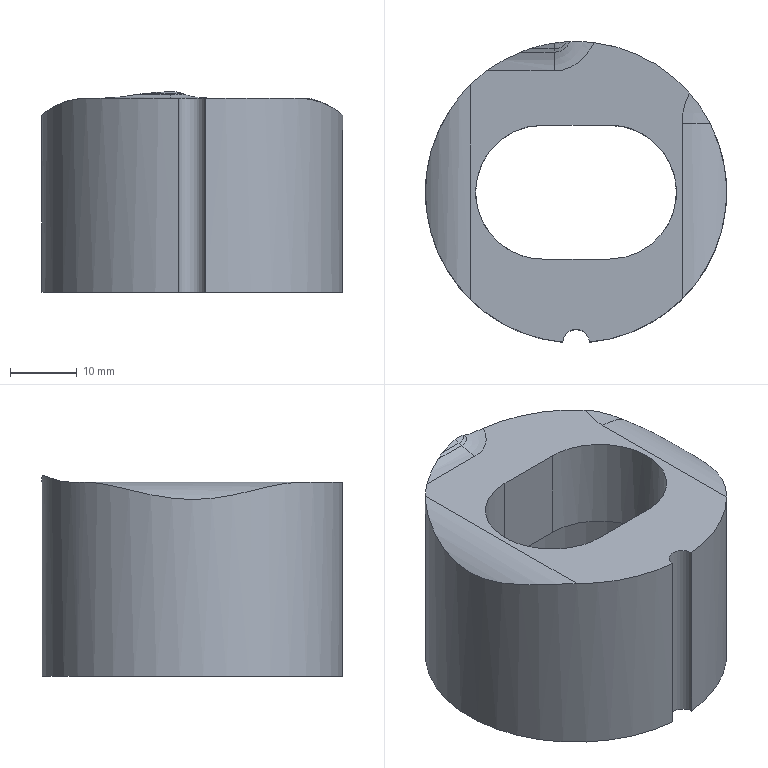Part | NX | features solid 2 | 1 solid | 19 faces | box 45 x 44.911 x 29.98 mm | volume 23323 mm3 | cylinder 10 | plane 6 | spline 3 | commonest cylinder face diameters 20 x3 12 x2 4 x1 15.009 x1 20.004 x1 36 x1
STEP:
#1=CARTESIAN_POINT('',(615.,-208.,21.));
#2=VERTEX_POINT('',#1);
#3=CARTESIAN_POINT('',(615.,-208.,35.));
#4=VERTEX_POINT('',#3);
#5=CARTESIAN_POINT('',(615.,-208.,-244.));
#6=DIRECTION('',(0.,0.,1.));
#7=VECTOR('',#6,1000.);
#8=LINE('',#5,#7);
#9=EDGE_CURVE('',#2,#4,#8,.T.);
#10=ORIENTED_EDGE('',*,*,#9,.T.);
#11=CARTESIAN_POINT('',(625.,-208.,35.));
#12=VERTEX_POINT('',#11);
#13=CARTESIAN_POINT('',(615.,-208.,35.));
#14=CARTESIAN_POINT('',(618.333,-208.,35.));
#15=CARTESIAN_POINT('',(621.666,-208.,35.));
#16=CARTESIAN_POINT('',(625.,-208.,35.));
#17=B_SPLINE_CURVE_WITH_KNOTS('',3,(#13,#14,#15,#16),.UNSPECIFIED.,.F.,.F.,(4,4),(0.,1.),.UNSPECIFIED.);
#18=EDGE_CURVE('',#4,#12,#17,.T.);
#19=ORIENTED_EDGE('',*,*,#18,.T.);
#20=CARTESIAN_POINT('',(625.,-208.,21.));
#21=VERTEX_POINT('',#20);
#22=CARTESIAN_POINT('',(625.,-208.,-244.));
#23=DIRECTION('',(0.,0.,1.));
#24=VECTOR('',#23,1000.);
#25=LINE('',#22,#24);
#26=EDGE_CURVE('',#21,#12,#25,.T.);
#27=ORIENTED_EDGE('',*,*,#26,.F.);
#28=CARTESIAN_POINT('',(615.,-208.,21.));
#29=DIRECTION('',(-1.,0.,0.));
#30=VECTOR('',#29,1000.);
#31=LINE('',#28,#30);
#32=EDGE_CURVE('',#21,#2,#31,.T.);
#33=ORIENTED_EDGE('',*,*,#32,.T.);
#34=EDGE_LOOP('',(#10,#19,#27,#33));
#35=FACE_BOUND('',#34,.T.);
#36=CARTESIAN_POINT('',(615.,-208.,-244.));
#37=DIRECTION('',(0.,1.,0.));
#38=DIRECTION('',(0.,0.,1.));
#39=AXIS2_PLACEMENT_3D('',#36,#37,#38);
#40=PLANE('',#39);
#41=ADVANCED_FACE('',(#35),#40,.T.);
#42=CARTESIAN_POINT('',(625.,-188.,35.));
#43=VERTEX_POINT('',#42);
#44=CARTESIAN_POINT('',(625.,-208.,35.));
#45=CARTESIAN_POINT('',(625.109,-207.999,35.));
#46=CARTESIAN_POINT('',(625.233,-207.998,35.));
#47=CARTESIAN_POINT('',(625.579,-207.987,35.));
#48=CARTESIAN_POINT('',(626.137,-207.945,35.));
#49=CARTESIAN_POINT('',(626.956,-207.826,35.));
#50=CARTESIAN_POINT('',(627.896,-207.589,35.));
#51=CARTESIAN_POINT('',(629.14,-207.143,35.));
#52=CARTESIAN_POINT('',(630.59,-206.373,35.));
#53=CARTESIAN_POINT('',(632.622,-204.701,35.));
#54=CARTESIAN_POINT('',(634.479,-201.929,35.));
#55=CARTESIAN_POINT('',(635.26,-198.,35.));
#56=CARTESIAN_POINT('',(634.479,-194.072,35.));
#57=CARTESIAN_POINT('',(632.622,-191.299,35.));
#58=CARTESIAN_POINT('',(630.591,-189.628,35.));
#59=CARTESIAN_POINT('',(629.14,-188.857,35.));
#60=CARTESIAN_POINT('',(627.898,-188.411,35.));
#61=CARTESIAN_POINT('',(626.956,-188.174,35.));
#62=CARTESIAN_POINT('',(626.137,-188.055,35.));
#63=CARTESIAN_POINT('',(625.579,-188.013,35.));
#64=CARTESIAN_POINT('',(625.233,-188.004,35.));
#65=CARTESIAN_POINT('',(625.109,-188.002,35.));
#66=CARTESIAN_POINT('',(625.,-188.,35.));
#67=B_SPLINE_CURVE_WITH_KNOTS('',3,(#44,#45,#46,#47,#48,#49,#50,#51,#52,#53,#54,#55,#56,#57,#58,#59,#60,#61,#62,#63,#64,#65,#66),.UNSPECIFIED.,.F.,.F.,(4,1,1,1,1,1,1,1,1,1,1,1,1,1,1,1,1,1,1,1,4),(0.,0.007812,0.01562,0.03125,0.0625,0.09375,0.125,0.1875,0.25,0.375,0.5,0.625,0.75,0.8125,0.875,0.9062,0.9375,0.9687,0.9844,0.9922,1.),.UNSPECIFIED.);
#68=EDGE_CURVE('',#43,#12,#67,.F.);
#69=ORIENTED_EDGE('',*,*,#68,.F.);
#70=CARTESIAN_POINT('',(625.,-188.,21.));
#71=VERTEX_POINT('',#70);
#72=CARTESIAN_POINT('',(625.,-188.,-244.));
#73=DIRECTION('',(0.,0.,1.));
#74=VECTOR('',#73,1000.);
#75=LINE('',#72,#74);
#76=EDGE_CURVE('',#71,#43,#75,.T.);
#77=ORIENTED_EDGE('',*,*,#76,.F.);
#78=CARTESIAN_POINT('',(625.,-198.,21.));
#79=DIRECTION('',(0.,0.,-1.));
#80=DIRECTION('',(-1.,0.,0.));
#81=AXIS2_PLACEMENT_3D('',#78,#79,#80);
#82=CIRCLE('',#81,10.);
#83=EDGE_CURVE('',#21,#71,#82,.F.);
#84=ORIENTED_EDGE('',*,*,#83,.F.);
#85=ORIENTED_EDGE('',*,*,#26,.T.);
#86=EDGE_LOOP('',(#69,#77,#84,#85));
#87=FACE_BOUND('',#86,.T.);
#88=CARTESIAN_POINT('',(625.,-198.,-244.));
#89=DIRECTION('',(0.,0.,1.));
#90=DIRECTION('',(-1.,0.,0.));
#91=AXIS2_PLACEMENT_3D('',#88,#89,#90);
#92=CYLINDRICAL_SURFACE('',#91,10.);
#93=ADVANCED_FACE('',(#87),#92,.F.);
#94=CARTESIAN_POINT('',(615.,-188.,35.));
#95=VERTEX_POINT('',#94);
#96=CARTESIAN_POINT('',(615.,-188.,35.));
#97=CARTESIAN_POINT('',(618.333,-188.,35.));
#98=CARTESIAN_POINT('',(621.666,-188.,35.));
#99=CARTESIAN_POINT('',(625.,-188.,35.));
#100=B_SPLINE_CURVE_WITH_KNOTS('',3,(#96,#97,#98,#99),.UNSPECIFIED.,.F.,.F.,(4,4),(0.,1.),.UNSPECIFIED.);
#101=EDGE_CURVE('',#95,#43,#100,.T.);
#102=ORIENTED_EDGE('',*,*,#101,.F.);
#103=CARTESIAN_POINT('',(615.,-188.,21.));
#104=VERTEX_POINT('',#103);
#105=CARTESIAN_POINT('',(615.,-188.,-244.));
#106=DIRECTION('',(0.,0.,1.));
#107=VECTOR('',#106,1000.);
#108=LINE('',#105,#107);
#109=EDGE_CURVE('',#104,#95,#108,.T.);
#110=ORIENTED_EDGE('',*,*,#109,.F.);
#111=CARTESIAN_POINT('',(615.,-188.,21.));
#112=DIRECTION('',(-1.,0.,0.));
#113=VECTOR('',#112,1000.);
#114=LINE('',#111,#113);
#115=EDGE_CURVE('',#71,#104,#114,.T.);
#116=ORIENTED_EDGE('',*,*,#115,.F.);
#117=ORIENTED_EDGE('',*,*,#76,.T.);
#118=EDGE_LOOP('',(#102,#110,#116,#117));
#119=FACE_BOUND('',#118,.T.);
#120=CARTESIAN_POINT('',(615.,-188.,-244.));
#121=DIRECTION('',(0.,1.,0.));
#122=DIRECTION('',(0.,0.,1.));
#123=AXIS2_PLACEMENT_3D('',#120,#121,#122);
#124=PLANE('',#123);
#125=ADVANCED_FACE('',(#119),#124,.F.);
#126=CARTESIAN_POINT('',(615.,-188.,35.));
#127=CARTESIAN_POINT('',(614.891,-188.001,35.));
#128=CARTESIAN_POINT('',(614.767,-188.002,35.));
#129=CARTESIAN_POINT('',(614.421,-188.013,35.));
#130=CARTESIAN_POINT('',(613.863,-188.055,35.));
#131=CARTESIAN_POINT('',(613.044,-188.174,35.));
#132=CARTESIAN_POINT('',(612.103,-188.411,35.));
#133=CARTESIAN_POINT('',(610.859,-188.857,35.));
#134=CARTESIAN_POINT('',(609.41,-189.627,35.));
#135=CARTESIAN_POINT('',(607.377,-191.299,35.));
#136=CARTESIAN_POINT('',(605.521,-194.071,35.));
#137=CARTESIAN_POINT('',(604.74,-198.,35.));
#138=CARTESIAN_POINT('',(605.52,-201.928,35.));
#139=CARTESIAN_POINT('',(607.378,-204.701,35.));
#140=CARTESIAN_POINT('',(609.409,-206.372,35.));
#141=CARTESIAN_POINT('',(610.86,-207.143,35.));
#142=CARTESIAN_POINT('',(612.102,-207.589,35.));
#143=CARTESIAN_POINT('',(613.044,-207.826,35.));
#144=CARTESIAN_POINT('',(613.863,-207.945,35.));
#145=CARTESIAN_POINT('',(614.421,-207.987,35.));
#146=CARTESIAN_POINT('',(614.767,-207.996,35.));
#147=CARTESIAN_POINT('',(614.891,-207.998,35.));
#148=CARTESIAN_POINT('',(615.,-208.,35.));
#149=B_SPLINE_CURVE_WITH_KNOTS('',3,(#126,#127,#128,#129,#130,#131,#132,#133,#134,#135,#136,#137,#138,#139,#140,#141,#142,#143,#144,#145,#146,#147,#148),.UNSPECIFIED.,.F.,.F.,(4,1,1,1,1,1,1,1,1,1,1,1,1,1,1,1,1,1,1,1,4),(0.,0.007812,0.01562,0.03125,0.0625,0.09375,0.125,0.1875,0.25,0.375,0.5,0.625,0.75,0.8125,0.875,0.9062,0.9375,0.9687,0.9844,0.9922,1.),.UNSPECIFIED.);
#150=EDGE_CURVE('',#4,#95,#149,.F.);
#151=ORIENTED_EDGE('',*,*,#150,.F.);
#152=ORIENTED_EDGE('',*,*,#9,.F.);
#153=CARTESIAN_POINT('',(615.,-198.,21.));
#154=DIRECTION('',(0.,0.,-1.));
#155=DIRECTION('',(-1.,0.,0.));
#156=AXIS2_PLACEMENT_3D('',#153,#154,#155);
#157=CIRCLE('',#156,10.);
#158=EDGE_CURVE('',#104,#2,#157,.F.);
#159=ORIENTED_EDGE('',*,*,#158,.F.);
#160=ORIENTED_EDGE('',*,*,#109,.T.);
#161=EDGE_LOOP('',(#151,#152,#159,#160));
#162=FACE_BOUND('',#161,.T.);
#163=CARTESIAN_POINT('',(615.,-198.,-244.));
#164=DIRECTION('',(0.,0.,1.));
#165=DIRECTION('',(-1.,0.,0.));
#166=AXIS2_PLACEMENT_3D('',#163,#164,#165);
#167=CYLINDRICAL_SURFACE('',#166,10.);
#168=ADVANCED_FACE('',(#162),#167,.F.);
#169=CARTESIAN_POINT('',(618.002,-220.411,6.));
#170=VERTEX_POINT('',#169);
#171=CARTESIAN_POINT('',(621.998,-220.411,6.));
#172=VERTEX_POINT('',#171);
#173=CARTESIAN_POINT('',(620.,-198.,6.));
#174=DIRECTION('',(0.,0.,-1.));
#175=DIRECTION('',(-1.,0.,0.));
#176=AXIS2_PLACEMENT_3D('',#173,#174,#175);
#177=CIRCLE('',#176,22.5);
#178=EDGE_CURVE('',#170,#172,#177,.T.);
#179=ORIENTED_EDGE('',*,*,#178,.T.);
#180=CARTESIAN_POINT('',(620.,-220.5,6.));
#181=DIRECTION('',(0.,0.,-1.));
#182=DIRECTION('',(0.,1.,0.));
#183=AXIS2_PLACEMENT_3D('',#180,#181,#182);
#184=CIRCLE('',#183,2.);
#185=EDGE_CURVE('',#170,#172,#184,.T.);
#186=ORIENTED_EDGE('',*,*,#185,.F.);
#187=EDGE_LOOP('',(#179,#186));
#188=FACE_BOUND('',#187,.T.);
#189=CARTESIAN_POINT('',(602.,-198.,6.));
#190=VERTEX_POINT('',#189);
#191=CARTESIAN_POINT('',(620.,-198.,6.));
#192=DIRECTION('',(0.,0.,-1.));
#193=DIRECTION('',(-1.,0.,0.));
#194=AXIS2_PLACEMENT_3D('',#191,#192,#193);
#195=CIRCLE('',#194,18.);
#196=EDGE_CURVE('',#190,#190,#195,.F.);
#197=ORIENTED_EDGE('',*,*,#196,.T.);
#198=EDGE_LOOP('',(#197));
#199=FACE_BOUND('',#198,.T.);
#200=CARTESIAN_POINT('',(620.,-198.,6.));
#201=DIRECTION('',(0.,0.,1.));
#202=DIRECTION('',(-1.,0.,0.));
#203=AXIS2_PLACEMENT_3D('',#200,#201,#202);
#204=PLANE('',#203);
#205=ADVANCED_FACE('',(#188,#199),#204,.F.);
#206=CARTESIAN_POINT('',(636.941,-183.193,35.));
#207=VERTEX_POINT('',#206);
#208=CARTESIAN_POINT('',(640.057,-187.804,34.071));
#209=VERTEX_POINT('',#208);
#210=CARTESIAN_POINT('',(636.941,-183.193,35.));
#211=CARTESIAN_POINT('',(638.198,-184.631,35.));
#212=CARTESIAN_POINT('',(639.217,-186.152,34.461));
#213=CARTESIAN_POINT('',(640.057,-187.804,34.069));
#214=B_SPLINE_CURVE_WITH_KNOTS('',3,(#210,#211,#212,#213),.UNSPECIFIED.,.F.,.F.,(4,4),(0.,0.005644),.UNSPECIFIED.);
#215=EDGE_CURVE('',#207,#209,#214,.T.);
#216=ORIENTED_EDGE('',*,*,#215,.T.);
#217=CARTESIAN_POINT('',(635.855,-213.965,35.));
#218=VERTEX_POINT('',#217);
#219=CARTESIAN_POINT('',(640.057,-187.804,34.072));
#220=CARTESIAN_POINT('',(641.122,-189.898,33.578));
#221=CARTESIAN_POINT('',(642.209,-193.22,32.737));
#222=CARTESIAN_POINT('',(642.597,-198.006,32.381));
#223=CARTESIAN_POINT('',(642.208,-202.794,32.741));
#224=CARTESIAN_POINT('',(640.362,-208.398,34.158));
#225=CARTESIAN_POINT('',(637.569,-212.262,35.));
#226=CARTESIAN_POINT('',(635.855,-213.964,35.));
#227=B_SPLINE_CURVE_WITH_KNOTS('',3,(#219,#220,#221,#222,#223,#224,#225,#226),.UNSPECIFIED.,.F.,.F.,(4,1,1,1,1,4),(0.0003348,0.007451,0.01101,0.01457,0.02168,0.0288),.UNSPECIFIED.);
#228=EDGE_CURVE('',#209,#218,#227,.T.);
#229=ORIENTED_EDGE('',*,*,#228,.T.);
#230=CARTESIAN_POINT('',(621.998,-220.411,35.));
#231=VERTEX_POINT('',#230);
#232=CARTESIAN_POINT('',(620.,-198.,35.));
#233=DIRECTION('',(0.,0.,-1.));
#234=DIRECTION('',(-1.,0.,0.));
#235=AXIS2_PLACEMENT_3D('',#232,#233,#234);
#236=CIRCLE('',#235,22.5);
#237=EDGE_CURVE('',#231,#218,#236,.F.);
#238=ORIENTED_EDGE('',*,*,#237,.F.);
#239=CARTESIAN_POINT('',(621.998,-220.411,21.));
#240=DIRECTION('',(0.,0.,-1.));
#241=VECTOR('',#240,1000.);
#242=LINE('',#239,#241);
#243=EDGE_CURVE('',#172,#231,#242,.F.);
#244=ORIENTED_EDGE('',*,*,#243,.F.);
#245=ORIENTED_EDGE('',*,*,#178,.F.);
#246=CARTESIAN_POINT('',(618.002,-220.411,35.));
#247=VERTEX_POINT('',#246);
#248=CARTESIAN_POINT('',(618.002,-220.411,21.));
#249=DIRECTION('',(0.,0.,-1.));
#250=VECTOR('',#249,1000.);
#251=LINE('',#248,#250);
#252=EDGE_CURVE('',#247,#170,#251,.T.);
#253=ORIENTED_EDGE('',*,*,#252,.F.);
#254=CARTESIAN_POINT('',(604.208,-214.028,35.));
#255=VERTEX_POINT('',#254);
#256=CARTESIAN_POINT('',(620.,-198.,35.));
#257=DIRECTION('',(0.,0.,-1.));
#258=DIRECTION('',(-1.,0.,0.));
#259=AXIS2_PLACEMENT_3D('',#256,#257,#258);
#260=CIRCLE('',#259,22.5);
#261=EDGE_CURVE('',#255,#247,#260,.F.);
#262=ORIENTED_EDGE('',*,*,#261,.F.);
#263=CARTESIAN_POINT('',(604.208,-181.972,35.));
#264=VERTEX_POINT('',#263);
#265=CARTESIAN_POINT('',(604.208,-214.028,35.));
#266=CARTESIAN_POINT('',(602.043,-211.894,35.));
#267=CARTESIAN_POINT('',(599.551,-208.158,34.001));
#268=CARTESIAN_POINT('',(597.807,-202.515,32.71));
#269=CARTESIAN_POINT('',(597.347,-198.025,32.27));
#270=CARTESIAN_POINT('',(597.802,-193.506,32.705));
#271=CARTESIAN_POINT('',(599.546,-187.85,34.));
#272=CARTESIAN_POINT('',(602.043,-184.106,35.));
#273=CARTESIAN_POINT('',(604.208,-181.972,35.));
#274=B_SPLINE_CURVE_WITH_KNOTS('',3,(#265,#266,#267,#268,#269,#270,#271,#272,#273),.UNSPECIFIED.,.F.,.F.,(4,1,1,1,1,1,4),(0.,0.009016,0.01352,0.01803,0.02254,0.02705,0.03606),.UNSPECIFIED.);
#275=EDGE_CURVE('',#255,#264,#274,.T.);
#276=ORIENTED_EDGE('',*,*,#275,.T.);
#277=CARTESIAN_POINT('',(606.645,-179.892,35.));
#278=VERTEX_POINT('',#277);
#279=CARTESIAN_POINT('',(620.,-198.,35.));
#280=DIRECTION('',(0.,0.,-1.));
#281=DIRECTION('',(-1.,0.,0.));
#282=AXIS2_PLACEMENT_3D('',#279,#280,#281);
#283=CIRCLE('',#282,22.5);
#284=EDGE_CURVE('',#278,#264,#283,.F.);
#285=ORIENTED_EDGE('',*,*,#284,.F.);
#286=CARTESIAN_POINT('',(611.709,-177.083,35.546));
#287=VERTEX_POINT('',#286);
#288=CARTESIAN_POINT('',(611.709,-177.083,35.546));
#289=CARTESIAN_POINT('',(609.909,-177.797,35.258));
#290=CARTESIAN_POINT('',(608.225,-178.727,35.));
#291=CARTESIAN_POINT('',(606.645,-179.892,35.));
#292=B_SPLINE_CURVE_WITH_KNOTS('',3,(#288,#289,#290,#291),.UNSPECIFIED.,.F.,.F.,(4,4),(0.,0.005817),.UNSPECIFIED.);
#293=EDGE_CURVE('',#287,#278,#292,.T.);
#294=ORIENTED_EDGE('',*,*,#293,.F.);
#295=CARTESIAN_POINT('',(613.191,-176.555,35.731));
#296=VERTEX_POINT('',#295);
#297=CARTESIAN_POINT('',(611.709,-177.083,35.546));
#298=CARTESIAN_POINT('',(612.194,-176.891,35.624));
#299=CARTESIAN_POINT('',(612.688,-176.715,35.683));
#300=CARTESIAN_POINT('',(613.191,-176.555,35.731));
#301=B_SPLINE_CURVE_WITH_KNOTS('',3,(#297,#298,#299,#300),.UNSPECIFIED.,.F.,.F.,(4,4),(0.006984,0.008558),.UNSPECIFIED.);
#302=EDGE_CURVE('',#287,#296,#301,.T.);
#303=ORIENTED_EDGE('',*,*,#302,.T.);
#304=CARTESIAN_POINT('',(616.734,-175.738,35.975));
#305=VERTEX_POINT('',#304);
#306=CARTESIAN_POINT('',(620.,-198.,29.318));
#307=DIRECTION('',(0.,-0.2865,0.9581));
#308=DIRECTION('',(0.,0.9581,0.2865));
#309=AXIS2_PLACEMENT_3D('',#306,#307,#308);
#310=ELLIPSE('',#309,23.485,22.5);
#311=EDGE_CURVE('',#296,#305,#310,.F.);
#312=ORIENTED_EDGE('',*,*,#311,.T.);
#313=CARTESIAN_POINT('',(618.619,-175.542,35.718));
#314=VERTEX_POINT('',#313);
#315=CARTESIAN_POINT('',(618.622,-175.542,35.716));
#316=CARTESIAN_POINT('',(618.016,-175.579,35.915));
#317=CARTESIAN_POINT('',(617.374,-175.644,36.003));
#318=CARTESIAN_POINT('',(616.734,-175.738,35.975));
#319=B_SPLINE_CURVE_WITH_KNOTS('',3,(#315,#316,#317,#318),.UNSPECIFIED.,.F.,.F.,(4,4),(0.002426,0.00434),.UNSPECIFIED.);
#320=EDGE_CURVE('',#314,#305,#319,.T.);
#321=ORIENTED_EDGE('',*,*,#320,.F.);
#322=CARTESIAN_POINT('',(619.085,-175.519,35.523));
#323=VERTEX_POINT('',#322);
#324=CARTESIAN_POINT('',(619.085,-175.519,35.523));
#325=CARTESIAN_POINT('',(618.927,-175.525,35.586));
#326=CARTESIAN_POINT('',(618.777,-175.533,35.666));
#327=CARTESIAN_POINT('',(618.617,-175.543,35.719));
#328=B_SPLINE_CURVE_WITH_KNOTS('',3,(#324,#325,#326,#327),.UNSPECIFIED.,.F.,.F.,(4,4),(0.,0.0005083),.UNSPECIFIED.);
#329=EDGE_CURVE('',#323,#314,#328,.T.);
#330=ORIENTED_EDGE('',*,*,#329,.F.);
#331=CARTESIAN_POINT('',(622.733,-175.667,35.));
#332=VERTEX_POINT('',#331);
#333=CARTESIAN_POINT('',(622.733,-175.667,35.));
#334=CARTESIAN_POINT('',(622.118,-175.591,35.));
#335=CARTESIAN_POINT('',(620.888,-175.492,35.073));
#336=CARTESIAN_POINT('',(619.655,-175.495,35.276));
#337=CARTESIAN_POINT('',(619.085,-175.519,35.523));
#338=B_SPLINE_CURVE_WITH_KNOTS('',3,(#333,#334,#335,#336,#337),.UNSPECIFIED.,.F.,.F.,(4,1,4),(0.,0.001854,0.003709),.UNSPECIFIED.);
#339=EDGE_CURVE('',#332,#323,#338,.T.);
#340=ORIENTED_EDGE('',*,*,#339,.F.);
#341=CARTESIAN_POINT('',(620.,-198.,35.));
#342=DIRECTION('',(0.,0.,-1.));
#343=DIRECTION('',(-1.,0.,0.));
#344=AXIS2_PLACEMENT_3D('',#341,#342,#343);
#345=CIRCLE('',#344,22.5);
#346=EDGE_CURVE('',#207,#332,#345,.F.);
#347=ORIENTED_EDGE('',*,*,#346,.F.);
#348=EDGE_LOOP('',(#216,#229,#238,#244,#245,#253,#262,#276,#285,#294,#303,#312,#321,#330,#340,#347));
#349=FACE_BOUND('',#348,.T.);
#350=CARTESIAN_POINT('',(620.,-198.,6.));
#351=DIRECTION('',(0.,0.,1.));
#352=DIRECTION('',(-1.,0.,0.));
#353=AXIS2_PLACEMENT_3D('',#350,#351,#352);
#354=CYLINDRICAL_SURFACE('',#353,22.5);
#355=ADVANCED_FACE('',(#349),#354,.T.);
#356=CARTESIAN_POINT('',(602.,-198.,21.));
#357=VERTEX_POINT('',#356);
#358=CARTESIAN_POINT('',(620.,-198.,21.));
#359=DIRECTION('',(0.,0.,-1.));
#360=DIRECTION('',(-1.,0.,0.));
#361=AXIS2_PLACEMENT_3D('',#358,#359,#360);
#362=CIRCLE('',#361,18.);
#363=EDGE_CURVE('',#357,#357,#362,.T.);
#364=ORIENTED_EDGE('',*,*,#363,.F.);
#365=EDGE_LOOP('',(#364));
#366=FACE_BOUND('',#365,.T.);
#367=ORIENTED_EDGE('',*,*,#196,.F.);
#368=EDGE_LOOP('',(#367));
#369=FACE_BOUND('',#368,.T.);
#370=CARTESIAN_POINT('',(620.,-198.,28.));
#371=DIRECTION('',(0.,0.,-1.));
#372=DIRECTION('',(1.,0.,0.));
#373=AXIS2_PLACEMENT_3D('',#370,#371,#372);
#374=CYLINDRICAL_SURFACE('',#373,18.);
#375=ADVANCED_FACE('',(#366,#369),#374,.F.);
#376=ORIENTED_EDGE('',*,*,#32,.F.);
#377=ORIENTED_EDGE('',*,*,#83,.T.);
#378=ORIENTED_EDGE('',*,*,#115,.T.);
#379=ORIENTED_EDGE('',*,*,#158,.T.);
#380=EDGE_LOOP('',(#376,#377,#378,#379));
#381=FACE_BOUND('',#380,.T.);
#382=ORIENTED_EDGE('',*,*,#363,.T.);
#383=EDGE_LOOP('',(#382));
#384=FACE_BOUND('',#383,.T.);
#385=CARTESIAN_POINT('',(620.,-198.,21.));
#386=DIRECTION('',(0.,0.,1.));
#387=DIRECTION('',(-1.,0.,0.));
#388=AXIS2_PLACEMENT_3D('',#385,#386,#387);
#389=PLANE('',#388);
#390=ADVANCED_FACE('',(#381,#384),#389,.F.);
#391=ORIENTED_EDGE('',*,*,#243,.T.);
#392=CARTESIAN_POINT('',(620.,-220.5,35.));
#393=DIRECTION('',(0.,0.,-1.));
#394=DIRECTION('',(-1.,0.,0.));
#395=AXIS2_PLACEMENT_3D('',#392,#393,#394);
#396=CIRCLE('',#395,2.);
#397=EDGE_CURVE('',#231,#247,#396,.F.);
#398=ORIENTED_EDGE('',*,*,#397,.T.);
#399=ORIENTED_EDGE('',*,*,#252,.T.);
#400=ORIENTED_EDGE('',*,*,#185,.T.);
#401=EDGE_LOOP('',(#391,#398,#399,#400));
#402=FACE_BOUND('',#401,.T.);
#403=CARTESIAN_POINT('',(620.,-220.5,36.));
#404=DIRECTION('',(0.,0.,-1.));
#405=DIRECTION('',(0.,-1.,0.));
#406=AXIS2_PLACEMENT_3D('',#403,#404,#405);
#407=CYLINDRICAL_SURFACE('',#406,2.);
#408=ADVANCED_FACE('',(#402),#407,.F.);
#409=CARTESIAN_POINT('',(616.734,-176.555,35.731));
#410=VERTEX_POINT('',#409);
#411=CARTESIAN_POINT('',(613.191,-176.555,35.731));
#412=CARTESIAN_POINT('',(614.372,-176.555,35.731));
#413=CARTESIAN_POINT('',(615.553,-176.555,35.731));
#414=CARTESIAN_POINT('',(616.734,-176.555,35.731));
#415=B_SPLINE_CURVE_WITH_KNOTS('',3,(#411,#412,#413,#414),.UNSPECIFIED.,.F.,.F.,(4,4),(0.8957,1.),.UNSPECIFIED.);
#416=EDGE_CURVE('',#410,#296,#415,.F.);
#417=ORIENTED_EDGE('',*,*,#416,.F.);
#418=CARTESIAN_POINT('',(616.734,-176.555,35.731));
#419=CARTESIAN_POINT('',(616.734,-176.283,35.813));
#420=CARTESIAN_POINT('',(616.734,-176.01,35.894));
#421=CARTESIAN_POINT('',(616.734,-175.738,35.975));
#422=B_SPLINE_CURVE_WITH_KNOTS('',3,(#418,#419,#420,#421),.UNSPECIFIED.,.F.,.F.,(4,4),(0.,0.03327),.UNSPECIFIED.);
#423=EDGE_CURVE('',#305,#410,#422,.F.);
#424=ORIENTED_EDGE('',*,*,#423,.F.);
#425=ORIENTED_EDGE('',*,*,#311,.F.);
#426=EDGE_LOOP('',(#417,#424,#425));
#427=FACE_BOUND('',#426,.T.);
#428=CARTESIAN_POINT('',(624.826,-176.555,35.731));
#429=DIRECTION('',(0.,-0.2865,0.9581));
#430=DIRECTION('',(0.,0.9581,0.2865));
#431=AXIS2_PLACEMENT_3D('',#428,#429,#430);
#432=PLANE('',#431);
#433=ADVANCED_FACE('',(#427),#432,.T.);
#434=ORIENTED_EDGE('',*,*,#320,.T.);
#435=ORIENTED_EDGE('',*,*,#423,.T.);
#436=CARTESIAN_POINT('',(616.734,-176.555,35.731));
#437=CARTESIAN_POINT('',(617.178,-176.555,35.731));
#438=CARTESIAN_POINT('',(617.933,-176.39,35.683));
#439=CARTESIAN_POINT('',(618.466,-175.808,35.69));
#440=CARTESIAN_POINT('',(618.621,-175.543,35.716));
#441=B_SPLINE_CURVE_WITH_KNOTS('',3,(#436,#437,#438,#439,#440),.UNSPECIFIED.,.F.,.F.,(4,1,4),(0.,0.1337,0.2675),.UNSPECIFIED.);
#442=EDGE_CURVE('',#410,#314,#441,.T.);
#443=ORIENTED_EDGE('',*,*,#442,.T.);
#444=EDGE_LOOP('',(#434,#435,#443));
#445=FACE_BOUND('',#444,.T.);
#446=CARTESIAN_POINT('',(616.734,-152.201,36.752));
#447=DIRECTION('',(0.,0.9581,0.2865));
#448=DIRECTION('',(0.,0.2865,-0.9581));
#449=AXIS2_PLACEMENT_3D('',#446,#447,#448);
#450=CYLINDRICAL_SURFACE('',#449,6.);
#451=ADVANCED_FACE('',(#445),#450,.T.);
#452=CARTESIAN_POINT('',(616.734,-177.083,35.546));
#453=VERTEX_POINT('',#452);
#454=CARTESIAN_POINT('',(611.709,-177.083,35.546));
#455=CARTESIAN_POINT('',(613.384,-177.083,35.546));
#456=CARTESIAN_POINT('',(615.059,-177.083,35.546));
#457=CARTESIAN_POINT('',(616.734,-177.083,35.546));
#458=B_SPLINE_CURVE_WITH_KNOTS('',3,(#454,#455,#456,#457),.UNSPECIFIED.,.F.,.F.,(4,4),(0.5988,1.),.UNSPECIFIED.);
#459=EDGE_CURVE('',#287,#453,#458,.T.);
#460=ORIENTED_EDGE('',*,*,#459,.T.);
#461=CARTESIAN_POINT('',(616.734,-177.083,35.546));
#462=CARTESIAN_POINT('',(616.734,-176.91,35.616));
#463=CARTESIAN_POINT('',(616.734,-176.734,35.678));
#464=CARTESIAN_POINT('',(616.734,-176.555,35.731));
#465=B_SPLINE_CURVE_WITH_KNOTS('',3,(#461,#462,#463,#464),.UNSPECIFIED.,.F.,.F.,(4,4),(0.,1.),.UNSPECIFIED.);
#466=EDGE_CURVE('',#453,#410,#465,.T.);
#467=ORIENTED_EDGE('',*,*,#466,.T.);
#468=ORIENTED_EDGE('',*,*,#416,.T.);
#469=ORIENTED_EDGE('',*,*,#302,.F.);
#470=EDGE_LOOP('',(#460,#467,#468,#469));
#471=FACE_BOUND('',#470,.T.);
#472=CARTESIAN_POINT('',(612.657,-174.837,29.983));
#473=DIRECTION('',(1.,0.,0.));
#474=DIRECTION('',(0.,1.,0.));
#475=AXIS2_PLACEMENT_3D('',#472,#473,#474);
#476=CYLINDRICAL_SURFACE('',#475,6.);
#477=ADVANCED_FACE('',(#471),#476,.T.);
#478=ORIENTED_EDGE('',*,*,#329,.T.);
#479=ORIENTED_EDGE('',*,*,#442,.F.);
#480=ORIENTED_EDGE('',*,*,#466,.F.);
#481=CARTESIAN_POINT('',(621.378,-166.946,36.5));
#482=CARTESIAN_POINT('',(621.222,-167.427,36.5));
#483=CARTESIAN_POINT('',(620.928,-168.394,36.462));
#484=CARTESIAN_POINT('',(620.416,-170.338,36.272));
#485=CARTESIAN_POINT('',(620.023,-172.276,35.97));
#486=CARTESIAN_POINT('',(619.591,-174.193,35.673));
#487=CARTESIAN_POINT('',(619.205,-175.345,35.528));
#488=CARTESIAN_POINT('',(618.713,-176.207,35.475));
#489=CARTESIAN_POINT('',(618.189,-176.732,35.481));
#490=CARTESIAN_POINT('',(617.488,-177.029,35.527));
#491=CARTESIAN_POINT('',(616.984,-177.084,35.546));
#492=CARTESIAN_POINT('',(616.734,-177.083,35.546));
#493=B_SPLINE_CURVE_WITH_KNOTS('',3,(#481,#482,#483,#484,#485,#486,#487,#488,#489,#490,#491,#492),.UNSPECIFIED.,.F.,.F.,(4,1,1,1,1,1,1,1,1,4),(0.,0.125,0.25,0.5,0.625,0.75,0.8125,0.875,0.9375,1.),.UNSPECIFIED.);
#494=EDGE_CURVE('',#453,#323,#493,.F.);
#495=ORIENTED_EDGE('',*,*,#494,.T.);
#496=EDGE_LOOP('',(#478,#479,#480,#495));
#497=FACE_BOUND('',#496,.T.);
#498=CARTESIAN_POINT('',(619.093,-175.502,35.524));
#499=CARTESIAN_POINT('',(619.018,-175.313,35.608));
#500=CARTESIAN_POINT('',(618.963,-175.127,35.71));
#501=CARTESIAN_POINT('',(618.897,-174.937,35.793));
#502=CARTESIAN_POINT('',(619.084,-175.52,35.523));
#503=CARTESIAN_POINT('',(619.01,-175.331,35.607));
#504=CARTESIAN_POINT('',(618.956,-175.145,35.707));
#505=CARTESIAN_POINT('',(618.89,-174.955,35.791));
#506=CARTESIAN_POINT('',(618.969,-175.759,35.502));
#507=CARTESIAN_POINT('',(618.904,-175.57,35.583));
#508=CARTESIAN_POINT('',(618.857,-175.385,35.677));
#509=CARTESIAN_POINT('',(618.799,-175.195,35.756));
#510=CARTESIAN_POINT('',(618.713,-176.207,35.475));
#511=CARTESIAN_POINT('',(618.666,-176.022,35.55));
#512=CARTESIAN_POINT('',(618.631,-175.839,35.632));
#513=CARTESIAN_POINT('',(618.589,-175.652,35.701));
#514=CARTESIAN_POINT('',(618.189,-176.732,35.481));
#515=CARTESIAN_POINT('',(618.162,-176.554,35.551));
#516=CARTESIAN_POINT('',(618.142,-176.375,35.621));
#517=CARTESIAN_POINT('',(618.118,-176.194,35.68));
#518=CARTESIAN_POINT('',(617.488,-177.029,35.527));
#519=CARTESIAN_POINT('',(617.476,-176.855,35.597));
#520=CARTESIAN_POINT('',(617.465,-176.677,35.661));
#521=CARTESIAN_POINT('',(617.454,-176.498,35.715));
#522=CARTESIAN_POINT('',(616.984,-177.084,35.546));
#523=CARTESIAN_POINT('',(616.98,-176.911,35.616));
#524=CARTESIAN_POINT('',(616.976,-176.734,35.678));
#525=CARTESIAN_POINT('',(616.972,-176.555,35.731));
#526=CARTESIAN_POINT('',(616.734,-177.083,35.546));
#527=CARTESIAN_POINT('',(616.734,-176.91,35.616));
#528=CARTESIAN_POINT('',(616.734,-176.734,35.678));
#529=CARTESIAN_POINT('',(616.734,-176.555,35.731));
#530=B_SPLINE_SURFACE_WITH_KNOTS('',3,3,((#498,#499,#500,#501),(#502,#503,#504,#505),(#506,#507,#508,#509),(#510,#511,#512,#513),(#514,#515,#516,#517),(#518,#519,#520,#521),(#522,#523,#524,#525),(#526,#527,#528,#529)),.UNSPECIFIED.,.F.,.F.,.F.,(4,1,1,1,1,4),(4,4),(0.745,0.75,0.8125,0.875,0.9375,1.),(0.,1.),.UNSPECIFIED.);
#531=ADVANCED_FACE('',(#497),#530,.F.);
#532=CARTESIAN_POINT('',(604.208,-214.028,35.));
#533=CARTESIAN_POINT('',(604.208,-203.343,35.));
#534=CARTESIAN_POINT('',(604.208,-192.657,35.));
#535=CARTESIAN_POINT('',(604.208,-181.972,35.));
#536=B_SPLINE_CURVE_WITH_KNOTS('',3,(#532,#533,#534,#535),.UNSPECIFIED.,.F.,.F.,(4,4),(0.3428,0.96),.UNSPECIFIED.);
#537=EDGE_CURVE('',#255,#264,#536,.T.);
#538=ORIENTED_EDGE('',*,*,#537,.T.);
#539=ORIENTED_EDGE('',*,*,#275,.F.);
#540=EDGE_LOOP('',(#538,#539));
#541=FACE_BOUND('',#540,.T.);
#542=CARTESIAN_POINT('',(604.208,-221.762,25.));
#543=DIRECTION('',(0.,-1.,0.));
#544=DIRECTION('',(1.,0.,0.));
#545=AXIS2_PLACEMENT_3D('',#542,#543,#544);
#546=CYLINDRICAL_SURFACE('',#545,10.);
#547=ADVANCED_FACE('',(#541),#546,.T.);
#548=ORIENTED_EDGE('',*,*,#293,.T.);
#549=CARTESIAN_POINT('',(616.734,-179.892,35.));
#550=VERTEX_POINT('',#549);
#551=CARTESIAN_POINT('',(606.645,-179.892,35.));
#552=CARTESIAN_POINT('',(610.008,-179.892,35.));
#553=CARTESIAN_POINT('',(613.371,-179.892,35.));
#554=CARTESIAN_POINT('',(616.734,-179.892,35.));
#555=B_SPLINE_CURVE_WITH_KNOTS('',3,(#551,#552,#553,#554),.UNSPECIFIED.,.F.,.F.,(4,4),(0.1945,1.),.UNSPECIFIED.);
#556=EDGE_CURVE('',#278,#550,#555,.T.);
#557=ORIENTED_EDGE('',*,*,#556,.T.);
#558=CARTESIAN_POINT('',(616.734,-177.083,35.546));
#559=CARTESIAN_POINT('',(616.734,-177.973,35.187));
#560=CARTESIAN_POINT('',(616.734,-178.933,35.));
#561=CARTESIAN_POINT('',(616.734,-179.892,35.));
#562=B_SPLINE_CURVE_WITH_KNOTS('',3,(#558,#559,#560,#561),.UNSPECIFIED.,.F.,.F.,(4,4),(0.,1.),.UNSPECIFIED.);
#563=EDGE_CURVE('',#550,#453,#562,.F.);
#564=ORIENTED_EDGE('',*,*,#563,.T.);
#565=ORIENTED_EDGE('',*,*,#459,.F.);
#566=EDGE_LOOP('',(#548,#557,#564,#565));
#567=FACE_BOUND('',#566,.T.);
#568=CARTESIAN_POINT('',(606.714,-179.894,42.505));
#569=DIRECTION('',(-1.,0.,0.));
#570=DIRECTION('',(0.,-1.,0.));
#571=AXIS2_PLACEMENT_3D('',#568,#569,#570);
#572=CYLINDRICAL_SURFACE('',#571,7.505);
#573=ADVANCED_FACE('',(#567),#572,.F.);
#574=ORIENTED_EDGE('',*,*,#339,.T.);
#575=ORIENTED_EDGE('',*,*,#494,.F.);
#576=ORIENTED_EDGE('',*,*,#563,.F.);
#577=CARTESIAN_POINT('',(616.734,-179.892,35.));
#578=CARTESIAN_POINT('',(616.948,-179.89,35.));
#579=CARTESIAN_POINT('',(617.193,-179.881,35.));
#580=CARTESIAN_POINT('',(617.872,-179.804,35.));
#581=CARTESIAN_POINT('',(618.638,-179.607,35.));
#582=CARTESIAN_POINT('',(619.524,-179.212,35.));
#583=CARTESIAN_POINT('',(620.34,-178.656,35.));
#584=CARTESIAN_POINT('',(621.004,-178.057,35.));
#585=CARTESIAN_POINT('',(621.914,-177.015,35.));
#586=CARTESIAN_POINT('',(622.406,-176.247,35.));
#587=CARTESIAN_POINT('',(622.735,-175.667,35.));
#588=B_SPLINE_CURVE_WITH_KNOTS('',3,(#577,#578,#579,#580,#581,#582,#583,#584,#585,#586,#587),.UNSPECIFIED.,.F.,.F.,(4,1,1,1,1,1,1,1,4),(0.,0.03091,0.06182,0.1236,0.1855,0.2473,0.3091,0.3709,0.4946),.UNSPECIFIED.);
#589=EDGE_CURVE('',#550,#332,#588,.T.);
#590=ORIENTED_EDGE('',*,*,#589,.T.);
#591=EDGE_LOOP('',(#574,#575,#576,#590));
#592=FACE_BOUND('',#591,.T.);
#593=CARTESIAN_POINT('',(622.756,-175.626,35.));
#594=CARTESIAN_POINT('',(621.767,-174.654,35.));
#595=CARTESIAN_POINT('',(620.702,-173.661,35.203));
#596=CARTESIAN_POINT('',(619.905,-172.785,35.891));
#597=CARTESIAN_POINT('',(622.442,-176.183,35.));
#598=CARTESIAN_POINT('',(621.527,-175.182,35.));
#599=CARTESIAN_POINT('',(620.538,-174.161,35.169));
#600=CARTESIAN_POINT('',(619.802,-173.256,35.818));
#601=CARTESIAN_POINT('',(621.744,-177.283,35.));
#602=CARTESIAN_POINT('',(620.996,-176.231,35.));
#603=CARTESIAN_POINT('',(620.186,-175.162,35.105));
#604=CARTESIAN_POINT('',(619.587,-174.203,35.671));
#605=CARTESIAN_POINT('',(620.636,-178.454,35.));
#606=CARTESIAN_POINT('',(620.136,-177.391,35.));
#607=CARTESIAN_POINT('',(619.6,-176.32,35.066));
#608=CARTESIAN_POINT('',(619.205,-175.345,35.528));
#609=CARTESIAN_POINT('',(619.553,-179.189,35.));
#610=CARTESIAN_POINT('',(619.256,-178.167,35.));
#611=CARTESIAN_POINT('',(618.944,-177.148,35.081));
#612=CARTESIAN_POINT('',(618.713,-176.207,35.475));
#613=CARTESIAN_POINT('',(618.663,-179.602,35.));
#614=CARTESIAN_POINT('',(618.492,-178.618,35.));
#615=CARTESIAN_POINT('',(618.319,-177.641,35.117));
#616=CARTESIAN_POINT('',(618.189,-176.732,35.481));
#617=CARTESIAN_POINT('',(617.712,-179.841,35.));
#618=CARTESIAN_POINT('',(617.631,-178.879,35.));
#619=CARTESIAN_POINT('',(617.551,-177.923,35.169));
#620=CARTESIAN_POINT('',(617.488,-177.029,35.527));
#621=CARTESIAN_POINT('',(617.06,-179.892,35.));
#622=CARTESIAN_POINT('',(617.032,-178.932,35.));
#623=CARTESIAN_POINT('',(617.005,-177.975,35.186));
#624=CARTESIAN_POINT('',(616.984,-177.084,35.546));
#625=CARTESIAN_POINT('',(616.734,-179.892,35.));
#626=CARTESIAN_POINT('',(616.734,-178.933,35.));
#627=CARTESIAN_POINT('',(616.734,-177.973,35.186));
#628=CARTESIAN_POINT('',(616.734,-177.083,35.546));
#629=B_SPLINE_SURFACE_WITH_KNOTS('',3,3,((#593,#594,#595,#596),(#597,#598,#599,#600),(#601,#602,#603,#604),(#605,#606,#607,#608),(#609,#610,#611,#612),(#613,#614,#615,#616),(#617,#618,#619,#620),(#621,#622,#623,#624),(#625,#626,#627,#628)),.UNSPECIFIED.,.F.,.F.,.F.,(4,1,1,1,1,1,4),(4,4),(0.5027,0.625,0.75,0.8125,0.875,0.9375,1.),(0.,1.),.UNSPECIFIED.);
#630=ADVANCED_FACE('',(#592),#629,.F.);
#631=CARTESIAN_POINT('',(635.852,-187.751,35.));
#632=VERTEX_POINT('',#631);
#633=CARTESIAN_POINT('',(636.941,-183.193,35.));
#634=CARTESIAN_POINT('',(636.76,-183.538,35.));
#635=CARTESIAN_POINT('',(636.434,-184.269,35.));
#636=CARTESIAN_POINT('',(636.093,-185.391,35.));
#637=CARTESIAN_POINT('',(635.924,-186.386,35.));
#638=CARTESIAN_POINT('',(635.868,-187.043,35.));
#639=CARTESIAN_POINT('',(635.854,-187.463,35.));
#640=CARTESIAN_POINT('',(635.852,-187.619,35.));
#641=CARTESIAN_POINT('',(635.85,-187.751,35.));
#642=B_SPLINE_CURVE_WITH_KNOTS('',3,(#633,#634,#635,#636,#637,#638,#639,#640,#641),.UNSPECIFIED.,.F.,.F.,(4,1,1,1,1,1,4),(0.8094,0.857,0.9047,0.9523,0.9762,0.9881,1.),.UNSPECIFIED.);
#643=EDGE_CURVE('',#207,#632,#642,.T.);
#644=ORIENTED_EDGE('',*,*,#643,.T.);
#645=CARTESIAN_POINT('',(635.85,-187.751,35.));
#646=CARTESIAN_POINT('',(636.076,-187.751,35.));
#647=CARTESIAN_POINT('',(636.372,-187.752,34.991));
#648=CARTESIAN_POINT('',(637.124,-187.756,34.932));
#649=CARTESIAN_POINT('',(638.347,-187.768,34.729));
#650=CARTESIAN_POINT('',(639.408,-187.788,34.373));
#651=CARTESIAN_POINT('',(640.057,-187.804,34.072));
#652=B_SPLINE_CURVE_WITH_KNOTS('',3,(#645,#646,#647,#648,#649,#650,#651),.UNSPECIFIED.,.F.,.F.,(4,1,1,1,4),(0.,0.0691,0.1382,0.2764,0.5528),.UNSPECIFIED.);
#653=EDGE_CURVE('',#632,#209,#652,.T.);
#654=ORIENTED_EDGE('',*,*,#653,.T.);
#655=ORIENTED_EDGE('',*,*,#215,.F.);
#656=EDGE_LOOP('',(#644,#654,#655));
#657=FACE_BOUND('',#656,.T.);
#658=CARTESIAN_POINT('',(640.084,-187.804,34.057));
#659=CARTESIAN_POINT('',(639.837,-187.798,34.173));
#660=CARTESIAN_POINT('',(638.34,-187.765,34.805));
#661=CARTESIAN_POINT('',(636.893,-187.751,35.));
#662=CARTESIAN_POINT('',(635.85,-187.751,35.));
#663=CARTESIAN_POINT('',(640.082,-187.422,34.057));
#664=CARTESIAN_POINT('',(639.835,-187.41,34.173));
#665=CARTESIAN_POINT('',(638.339,-187.337,34.805));
#666=CARTESIAN_POINT('',(636.895,-187.274,35.));
#667=CARTESIAN_POINT('',(635.849,-187.234,35.));
#668=CARTESIAN_POINT('',(640.132,-186.675,34.05));
#669=CARTESIAN_POINT('',(639.886,-186.649,34.167));
#670=CARTESIAN_POINT('',(638.398,-186.491,34.801));
#671=CARTESIAN_POINT('',(636.968,-186.324,35.));
#672=CARTESIAN_POINT('',(635.923,-186.197,35.));
#673=CARTESIAN_POINT('',(640.375,-185.598,34.017));
#674=CARTESIAN_POINT('',(640.135,-185.55,34.137));
#675=CARTESIAN_POINT('',(638.686,-185.249,34.787));
#676=CARTESIAN_POINT('',(637.303,-184.915,35.));
#677=CARTESIAN_POINT('',(636.279,-184.646,35.));
#678=CARTESIAN_POINT('',(640.656,-184.928,33.982));
#679=CARTESIAN_POINT('',(640.424,-184.864,34.104));
#680=CARTESIAN_POINT('',(639.022,-184.467,34.772));
#681=CARTESIAN_POINT('',(637.692,-184.022,35.));
#682=CARTESIAN_POINT('',(636.697,-183.656,35.));
#683=CARTESIAN_POINT('',(640.83,-184.599,33.962));
#684=CARTESIAN_POINT('',(640.603,-184.527,34.086));
#685=CARTESIAN_POINT('',(639.229,-184.083,34.763));
#686=CARTESIAN_POINT('',(637.93,-183.582,35.));
#687=CARTESIAN_POINT('',(636.954,-183.168,35.));
#688=B_SPLINE_SURFACE_WITH_KNOTS('',3,3,((#658,#659,#660,#661,#662),(#663,#664,#665,#666,#667),(#668,#669,#670,#671,#672),(#673,#674,#675,#676,#677),(#678,#679,#680,#681,#682),(#683,#684,#685,#686,#687)),.UNSPECIFIED.,.F.,.F.,.F.,(4,1,1,4),(4,1,4),(0.,0.0625,0.125,0.1916),(0.401,0.5,1.),.UNSPECIFIED.);
#689=ADVANCED_FACE('',(#657),#688,.T.);
#690=ORIENTED_EDGE('',*,*,#653,.F.);
#691=CARTESIAN_POINT('',(635.854,-187.751,35.));
#692=CARTESIAN_POINT('',(635.854,-196.489,35.));
#693=CARTESIAN_POINT('',(635.854,-205.227,35.));
#694=CARTESIAN_POINT('',(635.854,-213.965,35.));
#695=B_SPLINE_CURVE_WITH_KNOTS('',3,(#691,#692,#693,#694),.UNSPECIFIED.,.F.,.F.,(4,4),(0.,0.6525),.UNSPECIFIED.);
#696=EDGE_CURVE('',#632,#218,#695,.T.);
#697=ORIENTED_EDGE('',*,*,#696,.T.);
#698=ORIENTED_EDGE('',*,*,#228,.F.);
#699=EDGE_LOOP('',(#690,#697,#698));
#700=FACE_BOUND('',#699,.T.);
#701=CARTESIAN_POINT('',(635.85,-195.349,24.999));
#702=DIRECTION('',(0.0002477,-1.,-0.00001719));
#703=DIRECTION('',(1.,0.0002477,0.));
#704=AXIS2_PLACEMENT_3D('',#701,#702,#703);
#705=CYLINDRICAL_SURFACE('',#704,10.002);
#706=ADVANCED_FACE('',(#700),#705,.T.);
#707=ORIENTED_EDGE('',*,*,#346,.T.);
#708=ORIENTED_EDGE('',*,*,#589,.F.);
#709=ORIENTED_EDGE('',*,*,#556,.F.);
#710=ORIENTED_EDGE('',*,*,#284,.T.);
#711=ORIENTED_EDGE('',*,*,#537,.F.);
#712=ORIENTED_EDGE('',*,*,#261,.T.);
#713=ORIENTED_EDGE('',*,*,#397,.F.);
#714=ORIENTED_EDGE('',*,*,#237,.T.);
#715=ORIENTED_EDGE('',*,*,#696,.F.);
#716=ORIENTED_EDGE('',*,*,#643,.F.);
#717=EDGE_LOOP('',(#707,#708,#709,#710,#711,#712,#713,#714,#715,#716));
#718=FACE_BOUND('',#717,.T.);
#719=ORIENTED_EDGE('',*,*,#68,.T.);
#720=ORIENTED_EDGE('',*,*,#18,.F.);
#721=ORIENTED_EDGE('',*,*,#150,.T.);
#722=ORIENTED_EDGE('',*,*,#101,.T.);
#723=EDGE_LOOP('',(#719,#720,#721,#722));
#724=FACE_BOUND('',#723,.T.);
#725=CARTESIAN_POINT('',(552.725,-187.,35.));
#726=DIRECTION('',(0.,0.,-1.));
#727=DIRECTION('',(0.,-1.,0.));
#728=AXIS2_PLACEMENT_3D('',#725,#726,#727);
#729=PLANE('',#728);
#730=ADVANCED_FACE('',(#718,#724),#729,.F.);
#731=CLOSED_SHELL('',(#41,#93,#125,#168,#205,#355,#375,#390,#408,#433,#451,#477,#531,#547,#573,#630,#689,#706,#730));
#732=MANIFOLD_SOLID_BREP('',#731);
#733=(LENGTH_UNIT()NAMED_UNIT(*)SI_UNIT(.MILLI.,.METRE.));
#734=UNCERTAINTY_MEASURE_WITH_UNIT(LENGTH_MEASURE(0.051),#733,'','');
#735=(NAMED_UNIT(*)PLANE_ANGLE_UNIT()SI_UNIT($,.RADIAN.));
#736=(NAMED_UNIT(*)SI_UNIT($,.STERADIAN.)SOLID_ANGLE_UNIT());
#737=(GEOMETRIC_REPRESENTATION_CONTEXT(3)GLOBAL_UNCERTAINTY_ASSIGNED_CONTEXT((#734))GLOBAL_UNIT_ASSIGNED_CONTEXT((#733,#735,#736))REPRESENTATION_CONTEXT('',''));
#738=ADVANCED_BREP_SHAPE_REPRESENTATION('',(#732),#737);